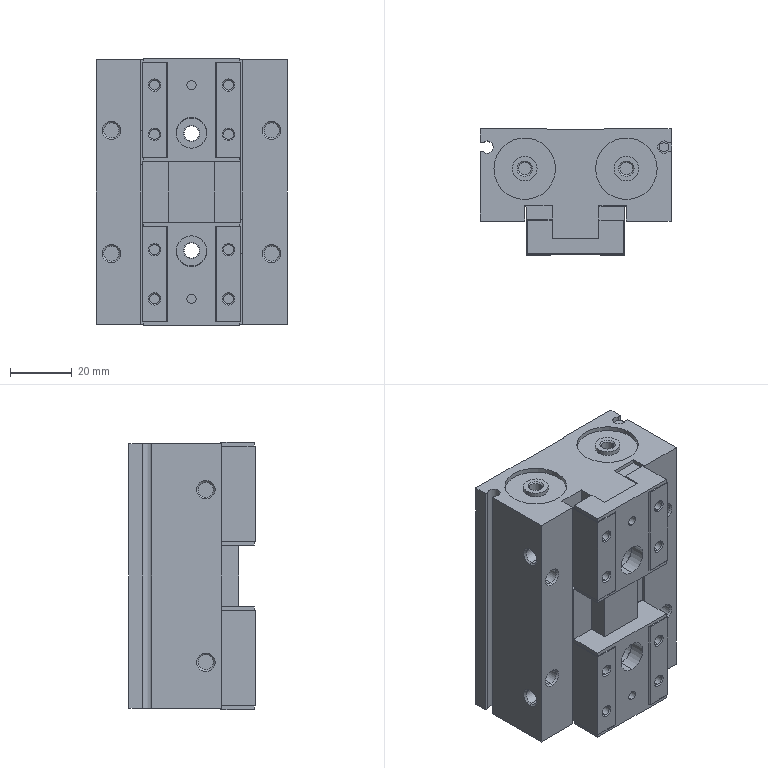Part | SolidWorks | 5 solids | 286 faces | box 62.3 x 41 x 86.8 mm | volume 172165 mm3 | plane 150 | cylinder 96 | cone 40 | commonest cylinder face diameters 4.917 x20 3.242 x16 4 x9 10 x8 20 x8 2.1 x6